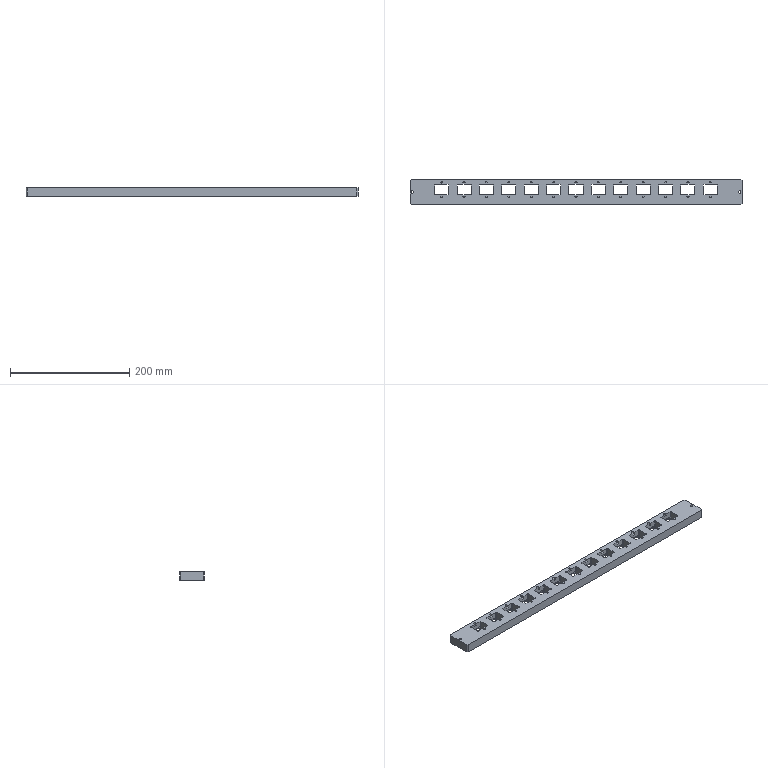NC program | NX | posted with a generic post | part box 556 x 41 x 15 mm
Lines 8982 to 9013 of 144595:
(ZLEVEL_PROFILE_COPY , TOOL : D10JING)
N17932 T11 M6
N17934 G54
N17936 G17 G0 G90 X-277.622 Y27.309 S5000 M3
N17938 G43 Z30. H11
N17940 Z-11.85
N17942 G94 G1 Z-14.85 F1000.
N17944 X-276.866 Y26.
N17946 G3 X-276. Y25.5 R1.
N17948 G1 X276.
N17950 G2 X279.536 Y24.036 R5.
N17952 G1 X281.536 Y22.036
N17954 G2 X283. Y18.5 R5.
N17956 G1 Y-18.5
N17958 G2 X281.536 Y-22.036 R5.
N17960 G1 X279.536 Y-24.036
N17962 G2 X276. Y-25.5 R5.
N17964 G1 X-276.
N17966 G2 X-279.536 Y-24.036 R5.
N17968 G1 X-281.536 Y-22.036
N17970 G2 X-283. Y-18.5 R5.
N17972 G1 Y18.5
N17974 G2 X-281.536 Y22.036 R5.
N17976 G1 X-279.536 Y24.036
N17978 G2 X-276. Y25.5 R5.
N17980 G3 X-275.134 Y26. R1.
N17982 G1 X-274.268 Y27.5
N17984 Z-11.85
N17986 G0 Z30.
N17988 M5